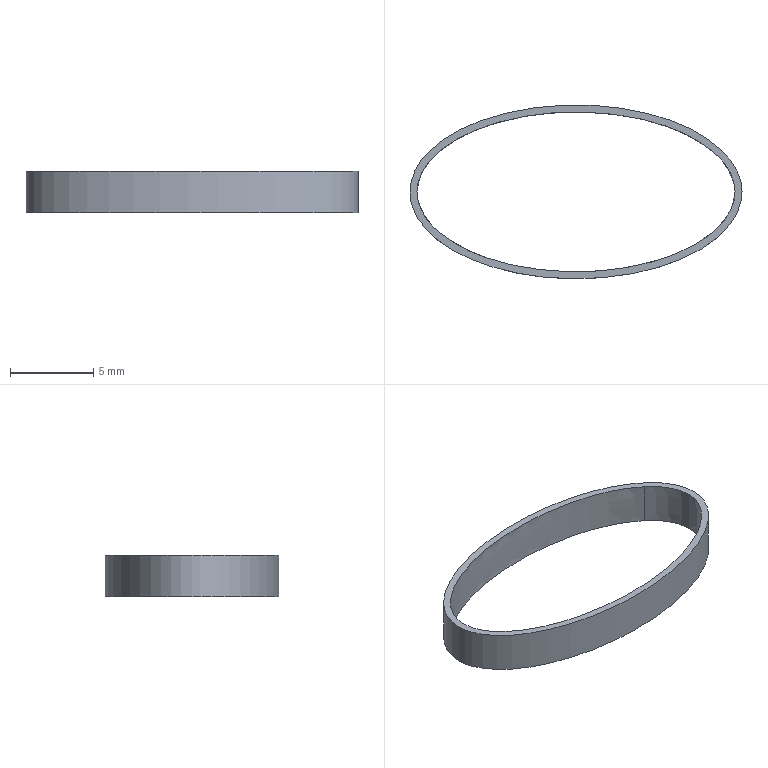Part | STEP file | lll_id1110_x_t | 1 solid | 9 faces | box 20 x 10.473 x 2.5 mm | volume 50.145 mm3 | other 7 | plane 2
STEP:
#1=CARTESIAN_POINT('',(381.689,-127.436,2.35));
#2=VERTEX_POINT('',#1);
#3=CARTESIAN_POINT('',(398.151,-127.436,2.35));
#4=VERTEX_POINT('',#3);
#5=CARTESIAN_POINT('',(381.689,-127.436,2.35));
#6=CARTESIAN_POINT('',(381.828,-127.553,2.35));
#7=CARTESIAN_POINT('',(381.971,-127.666,2.35));
#8=CARTESIAN_POINT('',(382.568,-128.082,2.35));
#9=CARTESIAN_POINT('',(383.043,-128.351,2.35));
#10=CARTESIAN_POINT('',(384.289,-128.906,2.35));
#11=CARTESIAN_POINT('',(385.064,-129.17,2.35));
#12=CARTESIAN_POINT('',(387.911,-129.83,2.35));
#13=CARTESIAN_POINT('',(390.012,-129.929,2.35));
#14=CARTESIAN_POINT('',(393.1,-129.572,2.35));
#15=CARTESIAN_POINT('',(394.082,-129.361,2.35));
#16=CARTESIAN_POINT('',(395.732,-128.839,2.35));
#17=CARTESIAN_POINT('',(396.4,-128.553,2.35));
#18=CARTESIAN_POINT('',(397.431,-127.982,2.35));
#19=CARTESIAN_POINT('',(397.804,-127.726,2.35));
#20=CARTESIAN_POINT('',(398.151,-127.436,2.35));
#21=(BOUNDED_CURVE()B_SPLINE_CURVE(3,(#5,#6,#7,#8,#9,#10,#11,#12,#13,#14,#15,#16,#17,#18,#19,#20),.UNSPECIFIED.,.F.,.F.)B_SPLINE_CURVE_WITH_KNOTS((4,2,2,2,2,2,2,4),(0.,0.03088,0.1235,0.2629,0.6224,0.7957,0.9214,1.),.UNSPECIFIED.)CURVE()GEOMETRIC_REPRESENTATION_ITEM()RATIONAL_B_SPLINE_CURVE((0.5011,0.5008,0.5008,0.4996,0.4996,0.4997,0.4997,0.4961,0.4961,0.4996,0.4996,0.4995,0.4995,0.4996,0.4996,0.5011))REPRESENTATION_ITEM(''));
#22=EDGE_CURVE('',#2,#4,#21,.T.);
#23=ORIENTED_EDGE('',*,*,#22,.T.);
#24=CARTESIAN_POINT('',(398.151,-127.436,-0.15));
#25=VERTEX_POINT('',#24);
#26=CARTESIAN_POINT('',(398.151,-127.436,-0.15));
#27=DIRECTION('',(0.,0.,1.));
#28=VECTOR('',#27,1.);
#29=LINE('',#26,#28);
#30=EDGE_CURVE('',#25,#4,#29,.T.);
#31=ORIENTED_EDGE('',*,*,#30,.F.);
#32=CARTESIAN_POINT('',(381.689,-127.436,-0.15));
#33=VERTEX_POINT('',#32);
#34=CARTESIAN_POINT('',(381.689,-127.436,-0.15));
#35=CARTESIAN_POINT('',(381.828,-127.553,-0.15));
#36=CARTESIAN_POINT('',(381.971,-127.666,-0.15));
#37=CARTESIAN_POINT('',(382.568,-128.082,-0.15));
#38=CARTESIAN_POINT('',(383.043,-128.351,-0.15));
#39=CARTESIAN_POINT('',(384.289,-128.906,-0.15));
#40=CARTESIAN_POINT('',(385.064,-129.17,-0.15));
#41=CARTESIAN_POINT('',(387.911,-129.83,-0.15));
#42=CARTESIAN_POINT('',(390.012,-129.929,-0.15));
#43=CARTESIAN_POINT('',(393.1,-129.572,-0.15));
#44=CARTESIAN_POINT('',(394.082,-129.361,-0.15));
#45=CARTESIAN_POINT('',(395.732,-128.839,-0.15));
#46=CARTESIAN_POINT('',(396.4,-128.553,-0.15));
#47=CARTESIAN_POINT('',(397.431,-127.982,-0.15));
#48=CARTESIAN_POINT('',(397.804,-127.726,-0.15));
#49=CARTESIAN_POINT('',(398.151,-127.436,-0.15));
#50=(BOUNDED_CURVE()B_SPLINE_CURVE(3,(#34,#35,#36,#37,#38,#39,#40,#41,#42,#43,#44,#45,#46,#47,#48,#49),.UNSPECIFIED.,.F.,.F.)B_SPLINE_CURVE_WITH_KNOTS((4,2,2,2,2,2,2,4),(0.,0.03088,0.1235,0.2629,0.6224,0.7957,0.9214,1.),.UNSPECIFIED.)CURVE()GEOMETRIC_REPRESENTATION_ITEM()RATIONAL_B_SPLINE_CURVE((0.5011,0.5008,0.5008,0.4996,0.4996,0.4997,0.4997,0.4961,0.4961,0.4996,0.4996,0.4995,0.4995,0.4996,0.4996,0.5011))REPRESENTATION_ITEM(''));
#51=EDGE_CURVE('',#33,#25,#50,.T.);
#52=ORIENTED_EDGE('',*,*,#51,.F.);
#53=CARTESIAN_POINT('',(381.689,-127.436,-0.15));
#54=DIRECTION('',(0.,0.,1.));
#55=VECTOR('',#54,1.);
#56=LINE('',#53,#55);
#57=EDGE_CURVE('',#33,#2,#56,.T.);
#58=ORIENTED_EDGE('',*,*,#57,.T.);
#59=EDGE_LOOP('',(#23,#31,#52,#58));
#60=FACE_OUTER_BOUND('',#59,.T.);
#61=CARTESIAN_POINT('',(381.689,-127.436,-0.15));
#62=CARTESIAN_POINT('',(381.828,-127.553,-0.15));
#63=CARTESIAN_POINT('',(381.971,-127.666,-0.15));
#64=CARTESIAN_POINT('',(382.568,-128.082,-0.15));
#65=CARTESIAN_POINT('',(383.043,-128.351,-0.15));
#66=CARTESIAN_POINT('',(384.289,-128.906,-0.15));
#67=CARTESIAN_POINT('',(385.064,-129.17,-0.15));
#68=CARTESIAN_POINT('',(387.911,-129.83,-0.15));
#69=CARTESIAN_POINT('',(390.012,-129.929,-0.15));
#70=CARTESIAN_POINT('',(393.1,-129.572,-0.15));
#71=CARTESIAN_POINT('',(394.082,-129.361,-0.15));
#72=CARTESIAN_POINT('',(395.732,-128.839,-0.15));
#73=CARTESIAN_POINT('',(396.4,-128.553,-0.15));
#74=CARTESIAN_POINT('',(397.431,-127.982,-0.15));
#75=CARTESIAN_POINT('',(397.804,-127.726,-0.15));
#76=CARTESIAN_POINT('',(398.151,-127.436,-0.15));
#77=(BOUNDED_CURVE()B_SPLINE_CURVE(3,(#61,#62,#63,#64,#65,#66,#67,#68,#69,#70,#71,#72,#73,#74,#75,#76),.UNSPECIFIED.,.F.,.F.)B_SPLINE_CURVE_WITH_KNOTS((4,2,2,2,2,2,2,4),(0.,0.03088,0.1235,0.2629,0.6224,0.7957,0.9214,1.),.UNSPECIFIED.)CURVE()GEOMETRIC_REPRESENTATION_ITEM()RATIONAL_B_SPLINE_CURVE((0.5011,0.5008,0.5008,0.4996,0.4996,0.4997,0.4997,0.4961,0.4961,0.4996,0.4996,0.4995,0.4995,0.4996,0.4996,0.5011))REPRESENTATION_ITEM(''));
#78=DIRECTION('',(0.,0.,1.));
#79=VECTOR('',#78,1.);
#80=SURFACE_OF_LINEAR_EXTRUSION('',#77,#79);
#81=ADVANCED_FACE('',(#60),#80,.F.);
#82=CARTESIAN_POINT('',(399.5,-125.,2.35));
#83=VERTEX_POINT('',#82);
#84=CARTESIAN_POINT('',(398.151,-127.436,2.35));
#85=CARTESIAN_POINT('',(398.314,-127.299,2.35));
#86=CARTESIAN_POINT('',(398.468,-127.152,2.35));
#87=CARTESIAN_POINT('',(398.795,-126.801,2.35));
#88=CARTESIAN_POINT('',(398.957,-126.589,2.35));
#89=CARTESIAN_POINT('',(399.188,-126.208,2.35));
#90=CARTESIAN_POINT('',(399.266,-126.048,2.35));
#91=CARTESIAN_POINT('',(399.443,-125.601,2.35));
#92=CARTESIAN_POINT('',(399.499,-125.303,2.35));
#93=CARTESIAN_POINT('',(399.5,-125.,2.35));
#94=(BOUNDED_CURVE()B_SPLINE_CURVE(3,(#84,#85,#86,#87,#88,#89,#90,#91,#92,#93),.UNSPECIFIED.,.F.,.F.)B_SPLINE_CURVE_WITH_KNOTS((4,2,2,2,4),(0.,0.2207,0.498,0.6834,1.),.UNSPECIFIED.)CURVE()GEOMETRIC_REPRESENTATION_ITEM()RATIONAL_B_SPLINE_CURVE((0.5044,0.5037,0.5037,0.5027,0.5027,0.5031,0.5031,0.4985,0.4985,0.5044))REPRESENTATION_ITEM(''));
#95=EDGE_CURVE('',#4,#83,#94,.T.);
#96=ORIENTED_EDGE('',*,*,#95,.T.);
#97=CARTESIAN_POINT('',(399.5,-125.,-0.15));
#98=VERTEX_POINT('',#97);
#99=CARTESIAN_POINT('',(399.5,-125.,-0.15));
#100=DIRECTION('',(0.,0.,1.));
#101=VECTOR('',#100,1.);
#102=LINE('',#99,#101);
#103=EDGE_CURVE('',#98,#83,#102,.T.);
#104=ORIENTED_EDGE('',*,*,#103,.F.);
#105=CARTESIAN_POINT('',(398.151,-127.436,-0.15));
#106=CARTESIAN_POINT('',(398.314,-127.299,-0.15));
#107=CARTESIAN_POINT('',(398.468,-127.152,-0.15));
#108=CARTESIAN_POINT('',(398.795,-126.801,-0.15));
#109=CARTESIAN_POINT('',(398.957,-126.589,-0.15));
#110=CARTESIAN_POINT('',(399.188,-126.208,-0.15));
#111=CARTESIAN_POINT('',(399.266,-126.048,-0.15));
#112=CARTESIAN_POINT('',(399.443,-125.601,-0.15));
#113=CARTESIAN_POINT('',(399.499,-125.303,-0.15));
#114=CARTESIAN_POINT('',(399.5,-125.,-0.15));
#115=(BOUNDED_CURVE()B_SPLINE_CURVE(3,(#105,#106,#107,#108,#109,#110,#111,#112,#113,#114),.UNSPECIFIED.,.F.,.F.)B_SPLINE_CURVE_WITH_KNOTS((4,2,2,2,4),(0.,0.2207,0.498,0.6834,1.),.UNSPECIFIED.)CURVE()GEOMETRIC_REPRESENTATION_ITEM()RATIONAL_B_SPLINE_CURVE((0.5044,0.5037,0.5037,0.5027,0.5027,0.5031,0.5031,0.4985,0.4985,0.5044))REPRESENTATION_ITEM(''));
#116=EDGE_CURVE('',#25,#98,#115,.T.);
#117=ORIENTED_EDGE('',*,*,#116,.F.);
#118=ORIENTED_EDGE('',*,*,#30,.T.);
#119=EDGE_LOOP('',(#96,#104,#117,#118));
#120=FACE_OUTER_BOUND('',#119,.T.);
#121=CARTESIAN_POINT('',(398.151,-127.436,-0.15));
#122=CARTESIAN_POINT('',(398.314,-127.299,-0.15));
#123=CARTESIAN_POINT('',(398.468,-127.152,-0.15));
#124=CARTESIAN_POINT('',(398.795,-126.801,-0.15));
#125=CARTESIAN_POINT('',(398.957,-126.589,-0.15));
#126=CARTESIAN_POINT('',(399.188,-126.208,-0.15));
#127=CARTESIAN_POINT('',(399.266,-126.048,-0.15));
#128=CARTESIAN_POINT('',(399.443,-125.601,-0.15));
#129=CARTESIAN_POINT('',(399.499,-125.303,-0.15));
#130=CARTESIAN_POINT('',(399.5,-125.,-0.15));
#131=(BOUNDED_CURVE()B_SPLINE_CURVE(3,(#121,#122,#123,#124,#125,#126,#127,#128,#129,#130),.UNSPECIFIED.,.F.,.F.)B_SPLINE_CURVE_WITH_KNOTS((4,2,2,2,4),(0.,0.2207,0.498,0.6834,1.),.UNSPECIFIED.)CURVE()GEOMETRIC_REPRESENTATION_ITEM()RATIONAL_B_SPLINE_CURVE((0.5044,0.5037,0.5037,0.5027,0.5027,0.5031,0.5031,0.4985,0.4985,0.5044))REPRESENTATION_ITEM(''));
#132=DIRECTION('',(0.,0.,1.));
#133=VECTOR('',#132,1.);
#134=SURFACE_OF_LINEAR_EXTRUSION('',#131,#133);
#135=ADVANCED_FACE('',(#120),#134,.F.);
#136=CARTESIAN_POINT('',(398.151,-122.564,2.35));
#137=VERTEX_POINT('',#136);
#138=CARTESIAN_POINT('',(399.5,-125.,2.35));
#139=CARTESIAN_POINT('',(399.499,-124.667,2.35));
#140=CARTESIAN_POINT('',(399.429,-124.341,2.35));
#141=CARTESIAN_POINT('',(399.24,-123.898,2.35));
#142=CARTESIAN_POINT('',(399.172,-123.766,2.35));
#143=CARTESIAN_POINT('',(398.972,-123.437,2.35));
#144=CARTESIAN_POINT('',(398.831,-123.247,2.35));
#145=CARTESIAN_POINT('',(398.512,-122.889,2.35));
#146=CARTESIAN_POINT('',(398.337,-122.72,2.35));
#147=CARTESIAN_POINT('',(398.151,-122.564,2.35));
#148=(BOUNDED_CURVE()B_SPLINE_CURVE(3,(#138,#139,#140,#141,#142,#143,#144,#145,#146,#147),.UNSPECIFIED.,.F.,.F.)B_SPLINE_CURVE_WITH_KNOTS((4,2,2,2,4),(0.,0.3431,0.4977,0.7454,1.),.UNSPECIFIED.)CURVE()GEOMETRIC_REPRESENTATION_ITEM()RATIONAL_B_SPLINE_CURVE((0.5007,0.4938,0.4938,0.4998,0.4998,0.4993,0.4993,0.4998,0.4998,0.5007))REPRESENTATION_ITEM(''));
#149=EDGE_CURVE('',#83,#137,#148,.T.);
#150=ORIENTED_EDGE('',*,*,#149,.T.);
#151=CARTESIAN_POINT('',(398.151,-122.564,-0.15));
#152=VERTEX_POINT('',#151);
#153=CARTESIAN_POINT('',(398.151,-122.564,-0.15));
#154=DIRECTION('',(0.,0.,1.));
#155=VECTOR('',#154,1.);
#156=LINE('',#153,#155);
#157=EDGE_CURVE('',#152,#137,#156,.T.);
#158=ORIENTED_EDGE('',*,*,#157,.F.);
#159=CARTESIAN_POINT('',(399.5,-125.,-0.15));
#160=CARTESIAN_POINT('',(399.499,-124.667,-0.15));
#161=CARTESIAN_POINT('',(399.429,-124.341,-0.15));
#162=CARTESIAN_POINT('',(399.24,-123.898,-0.15));
#163=CARTESIAN_POINT('',(399.172,-123.766,-0.15));
#164=CARTESIAN_POINT('',(398.972,-123.437,-0.15));
#165=CARTESIAN_POINT('',(398.831,-123.247,-0.15));
#166=CARTESIAN_POINT('',(398.512,-122.889,-0.15));
#167=CARTESIAN_POINT('',(398.337,-122.72,-0.15));
#168=CARTESIAN_POINT('',(398.151,-122.564,-0.15));
#169=(BOUNDED_CURVE()B_SPLINE_CURVE(3,(#159,#160,#161,#162,#163,#164,#165,#166,#167,#168),.UNSPECIFIED.,.F.,.F.)B_SPLINE_CURVE_WITH_KNOTS((4,2,2,2,4),(0.,0.3431,0.4977,0.7454,1.),.UNSPECIFIED.)CURVE()GEOMETRIC_REPRESENTATION_ITEM()RATIONAL_B_SPLINE_CURVE((0.5007,0.4938,0.4938,0.4998,0.4998,0.4993,0.4993,0.4998,0.4998,0.5007))REPRESENTATION_ITEM(''));
#170=EDGE_CURVE('',#98,#152,#169,.T.);
#171=ORIENTED_EDGE('',*,*,#170,.F.);
#172=ORIENTED_EDGE('',*,*,#103,.T.);
#173=EDGE_LOOP('',(#150,#158,#171,#172));
#174=FACE_OUTER_BOUND('',#173,.T.);
#175=CARTESIAN_POINT('',(399.5,-125.,-0.15));
#176=CARTESIAN_POINT('',(399.499,-124.667,-0.15));
#177=CARTESIAN_POINT('',(399.429,-124.341,-0.15));
#178=CARTESIAN_POINT('',(399.24,-123.898,-0.15));
#179=CARTESIAN_POINT('',(399.172,-123.766,-0.15));
#180=CARTESIAN_POINT('',(398.972,-123.437,-0.15));
#181=CARTESIAN_POINT('',(398.831,-123.247,-0.15));
#182=CARTESIAN_POINT('',(398.512,-122.889,-0.15));
#183=CARTESIAN_POINT('',(398.337,-122.72,-0.15));
#184=CARTESIAN_POINT('',(398.151,-122.564,-0.15));
#185=(BOUNDED_CURVE()B_SPLINE_CURVE(3,(#175,#176,#177,#178,#179,#180,#181,#182,#183,#184),.UNSPECIFIED.,.F.,.F.)B_SPLINE_CURVE_WITH_KNOTS((4,2,2,2,4),(0.,0.3431,0.4977,0.7454,1.),.UNSPECIFIED.)CURVE()GEOMETRIC_REPRESENTATION_ITEM()RATIONAL_B_SPLINE_CURVE((0.5007,0.4938,0.4938,0.4998,0.4998,0.4993,0.4993,0.4998,0.4998,0.5007))REPRESENTATION_ITEM(''));
#186=DIRECTION('',(0.,0.,1.));
#187=VECTOR('',#186,1.);
#188=SURFACE_OF_LINEAR_EXTRUSION('',#185,#187);
#189=ADVANCED_FACE('',(#174),#188,.F.);
#190=CARTESIAN_POINT('',(381.689,-122.564,2.35));
#191=VERTEX_POINT('',#190);
#192=CARTESIAN_POINT('',(398.151,-122.564,2.35));
#193=CARTESIAN_POINT('',(398.012,-122.447,2.35));
#194=CARTESIAN_POINT('',(397.869,-122.335,2.35));
#195=CARTESIAN_POINT('',(397.272,-121.918,2.35));
#196=CARTESIAN_POINT('',(396.797,-121.649,2.35));
#197=CARTESIAN_POINT('',(395.551,-121.094,2.35));
#198=CARTESIAN_POINT('',(394.776,-120.831,2.35));
#199=CARTESIAN_POINT('',(391.929,-120.17,2.35));
#200=CARTESIAN_POINT('',(389.828,-120.071,2.35));
#201=CARTESIAN_POINT('',(386.74,-120.428,2.35));
#202=CARTESIAN_POINT('',(385.758,-120.639,2.35));
#203=CARTESIAN_POINT('',(384.108,-121.162,2.35));
#204=CARTESIAN_POINT('',(383.44,-121.447,2.35));
#205=CARTESIAN_POINT('',(382.409,-122.018,2.35));
#206=CARTESIAN_POINT('',(382.036,-122.274,2.35));
#207=CARTESIAN_POINT('',(381.689,-122.564,2.35));
#208=(BOUNDED_CURVE()B_SPLINE_CURVE(3,(#192,#193,#194,#195,#196,#197,#198,#199,#200,#201,#202,#203,#204,#205,#206,#207),.UNSPECIFIED.,.F.,.F.)B_SPLINE_CURVE_WITH_KNOTS((4,2,2,2,2,2,2,4),(0.,0.03088,0.1235,0.2629,0.6224,0.7957,0.9214,1.),.UNSPECIFIED.)CURVE()GEOMETRIC_REPRESENTATION_ITEM()RATIONAL_B_SPLINE_CURVE((0.5011,0.5008,0.5008,0.4996,0.4996,0.4997,0.4997,0.4961,0.4961,0.4996,0.4996,0.4995,0.4995,0.4996,0.4996,0.5011))REPRESENTATION_ITEM(''));
#209=EDGE_CURVE('',#137,#191,#208,.T.);
#210=ORIENTED_EDGE('',*,*,#209,.T.);
#211=CARTESIAN_POINT('',(381.689,-122.564,-0.15));
#212=VERTEX_POINT('',#211);
#213=CARTESIAN_POINT('',(381.689,-122.564,-0.15));
#214=DIRECTION('',(0.,0.,1.));
#215=VECTOR('',#214,1.);
#216=LINE('',#213,#215);
#217=EDGE_CURVE('',#212,#191,#216,.T.);
#218=ORIENTED_EDGE('',*,*,#217,.F.);
#219=CARTESIAN_POINT('',(398.151,-122.564,-0.15));
#220=CARTESIAN_POINT('',(398.012,-122.447,-0.15));
#221=CARTESIAN_POINT('',(397.869,-122.335,-0.15));
#222=CARTESIAN_POINT('',(397.272,-121.918,-0.15));
#223=CARTESIAN_POINT('',(396.797,-121.649,-0.15));
#224=CARTESIAN_POINT('',(395.551,-121.094,-0.15));
#225=CARTESIAN_POINT('',(394.776,-120.831,-0.15));
#226=CARTESIAN_POINT('',(391.929,-120.17,-0.15));
#227=CARTESIAN_POINT('',(389.828,-120.071,-0.15));
#228=CARTESIAN_POINT('',(386.74,-120.428,-0.15));
#229=CARTESIAN_POINT('',(385.758,-120.639,-0.15));
#230=CARTESIAN_POINT('',(384.108,-121.162,-0.15));
#231=CARTESIAN_POINT('',(383.44,-121.447,-0.15));
#232=CARTESIAN_POINT('',(382.409,-122.018,-0.15));
#233=CARTESIAN_POINT('',(382.036,-122.274,-0.15));
#234=CARTESIAN_POINT('',(381.689,-122.564,-0.15));
#235=(BOUNDED_CURVE()B_SPLINE_CURVE(3,(#219,#220,#221,#222,#223,#224,#225,#226,#227,#228,#229,#230,#231,#232,#233,#234),.UNSPECIFIED.,.F.,.F.)B_SPLINE_CURVE_WITH_KNOTS((4,2,2,2,2,2,2,4),(0.,0.03088,0.1235,0.2629,0.6224,0.7957,0.9214,1.),.UNSPECIFIED.)CURVE()GEOMETRIC_REPRESENTATION_ITEM()RATIONAL_B_SPLINE_CURVE((0.5011,0.5008,0.5008,0.4996,0.4996,0.4997,0.4997,0.4961,0.4961,0.4996,0.4996,0.4995,0.4995,0.4996,0.4996,0.5011))REPRESENTATION_ITEM(''));
#236=EDGE_CURVE('',#152,#212,#235,.T.);
#237=ORIENTED_EDGE('',*,*,#236,.F.);
#238=ORIENTED_EDGE('',*,*,#157,.T.);
#239=EDGE_LOOP('',(#210,#218,#237,#238));
#240=FACE_OUTER_BOUND('',#239,.T.);
#241=CARTESIAN_POINT('',(398.151,-122.564,-0.15));
#242=CARTESIAN_POINT('',(398.012,-122.447,-0.15));
#243=CARTESIAN_POINT('',(397.869,-122.335,-0.15));
#244=CARTESIAN_POINT('',(397.272,-121.918,-0.15));
#245=CARTESIAN_POINT('',(396.797,-121.649,-0.15));
#246=CARTESIAN_POINT('',(395.551,-121.094,-0.15));
#247=CARTESIAN_POINT('',(394.776,-120.831,-0.15));
#248=CARTESIAN_POINT('',(391.929,-120.17,-0.15));
#249=CARTESIAN_POINT('',(389.828,-120.071,-0.15));
#250=CARTESIAN_POINT('',(386.74,-120.428,-0.15));
#251=CARTESIAN_POINT('',(385.758,-120.639,-0.15));
#252=CARTESIAN_POINT('',(384.108,-121.162,-0.15));
#253=CARTESIAN_POINT('',(383.44,-121.447,-0.15));
#254=CARTESIAN_POINT('',(382.409,-122.018,-0.15));
#255=CARTESIAN_POINT('',(382.036,-122.274,-0.15));
#256=CARTESIAN_POINT('',(381.689,-122.564,-0.15));
#257=(BOUNDED_CURVE()B_SPLINE_CURVE(3,(#241,#242,#243,#244,#245,#246,#247,#248,#249,#250,#251,#252,#253,#254,#255,#256),.UNSPECIFIED.,.F.,.F.)B_SPLINE_CURVE_WITH_KNOTS((4,2,2,2,2,2,2,4),(0.,0.03088,0.1235,0.2629,0.6224,0.7957,0.9214,1.),.UNSPECIFIED.)CURVE()GEOMETRIC_REPRESENTATION_ITEM()RATIONAL_B_SPLINE_CURVE((0.5011,0.5008,0.5008,0.4996,0.4996,0.4997,0.4997,0.4961,0.4961,0.4996,0.4996,0.4995,0.4995,0.4996,0.4996,0.5011))REPRESENTATION_ITEM(''));
#258=DIRECTION('',(0.,0.,1.));
#259=VECTOR('',#258,1.);
#260=SURFACE_OF_LINEAR_EXTRUSION('',#257,#259);
#261=ADVANCED_FACE('',(#240),#260,.F.);
#262=CARTESIAN_POINT('',(380.34,-125.,2.35));
#263=VERTEX_POINT('',#262);
#264=CARTESIAN_POINT('',(381.689,-122.564,2.35));
#265=CARTESIAN_POINT('',(381.526,-122.701,2.35));
#266=CARTESIAN_POINT('',(381.372,-122.848,2.35));
#267=CARTESIAN_POINT('',(381.045,-123.199,2.35));
#268=CARTESIAN_POINT('',(380.883,-123.412,2.35));
#269=CARTESIAN_POINT('',(380.652,-123.792,2.35));
#270=CARTESIAN_POINT('',(380.574,-123.952,2.35));
#271=CARTESIAN_POINT('',(380.397,-124.399,2.35));
#272=CARTESIAN_POINT('',(380.341,-124.697,2.35));
#273=CARTESIAN_POINT('',(380.34,-125.,2.35));
#274=(BOUNDED_CURVE()B_SPLINE_CURVE(3,(#264,#265,#266,#267,#268,#269,#270,#271,#272,#273),.UNSPECIFIED.,.F.,.F.)B_SPLINE_CURVE_WITH_KNOTS((4,2,2,2,4),(0.,0.2207,0.498,0.6834,1.),.UNSPECIFIED.)CURVE()GEOMETRIC_REPRESENTATION_ITEM()RATIONAL_B_SPLINE_CURVE((0.5044,0.5037,0.5037,0.5027,0.5027,0.5031,0.5031,0.4985,0.4985,0.5044))REPRESENTATION_ITEM(''));
#275=EDGE_CURVE('',#191,#263,#274,.T.);
#276=ORIENTED_EDGE('',*,*,#275,.T.);
#277=CARTESIAN_POINT('',(380.34,-125.,-0.15));
#278=VERTEX_POINT('',#277);
#279=CARTESIAN_POINT('',(380.34,-125.,-0.15));
#280=DIRECTION('',(0.,0.,1.));
#281=VECTOR('',#280,1.);
#282=LINE('',#279,#281);
#283=EDGE_CURVE('',#278,#263,#282,.T.);
#284=ORIENTED_EDGE('',*,*,#283,.F.);
#285=CARTESIAN_POINT('',(381.689,-122.564,-0.15));
#286=CARTESIAN_POINT('',(381.526,-122.701,-0.15));
#287=CARTESIAN_POINT('',(381.372,-122.848,-0.15));
#288=CARTESIAN_POINT('',(381.045,-123.199,-0.15));
#289=CARTESIAN_POINT('',(380.883,-123.412,-0.15));
#290=CARTESIAN_POINT('',(380.652,-123.792,-0.15));
#291=CARTESIAN_POINT('',(380.574,-123.952,-0.15));
#292=CARTESIAN_POINT('',(380.397,-124.399,-0.15));
#293=CARTESIAN_POINT('',(380.341,-124.697,-0.15));
#294=CARTESIAN_POINT('',(380.34,-125.,-0.15));
#295=(BOUNDED_CURVE()B_SPLINE_CURVE(3,(#285,#286,#287,#288,#289,#290,#291,#292,#293,#294),.UNSPECIFIED.,.F.,.F.)B_SPLINE_CURVE_WITH_KNOTS((4,2,2,2,4),(0.,0.2207,0.498,0.6834,1.),.UNSPECIFIED.)CURVE()GEOMETRIC_REPRESENTATION_ITEM()RATIONAL_B_SPLINE_CURVE((0.5044,0.5037,0.5037,0.5027,0.5027,0.5031,0.5031,0.4985,0.4985,0.5044))REPRESENTATION_ITEM(''));
#296=EDGE_CURVE('',#212,#278,#295,.T.);
#297=ORIENTED_EDGE('',*,*,#296,.F.);
#298=ORIENTED_EDGE('',*,*,#217,.T.);
#299=EDGE_LOOP('',(#276,#284,#297,#298));
#300=FACE_OUTER_BOUND('',#299,.T.);
#301=CARTESIAN_POINT('',(381.689,-122.564,-0.15));
#302=CARTESIAN_POINT('',(381.526,-122.701,-0.15));
#303=CARTESIAN_POINT('',(381.372,-122.848,-0.15));
#304=CARTESIAN_POINT('',(381.045,-123.199,-0.15));
#305=CARTESIAN_POINT('',(380.883,-123.412,-0.15));
#306=CARTESIAN_POINT('',(380.652,-123.792,-0.15));
#307=CARTESIAN_POINT('',(380.574,-123.952,-0.15));
#308=CARTESIAN_POINT('',(380.397,-124.399,-0.15));
#309=CARTESIAN_POINT('',(380.341,-124.697,-0.15));
#310=CARTESIAN_POINT('',(380.34,-125.,-0.15));
#311=(BOUNDED_CURVE()B_SPLINE_CURVE(3,(#301,#302,#303,#304,#305,#306,#307,#308,#309,#310),.UNSPECIFIED.,.F.,.F.)B_SPLINE_CURVE_WITH_KNOTS((4,2,2,2,4),(0.,0.2207,0.498,0.6834,1.),.UNSPECIFIED.)CURVE()GEOMETRIC_REPRESENTATION_ITEM()RATIONAL_B_SPLINE_CURVE((0.5044,0.5037,0.5037,0.5027,0.5027,0.5031,0.5031,0.4985,0.4985,0.5044))REPRESENTATION_ITEM(''));
#312=DIRECTION('',(0.,0.,1.));
#313=VECTOR('',#312,1.);
#314=SURFACE_OF_LINEAR_EXTRUSION('',#311,#313);
#315=ADVANCED_FACE('',(#300),#314,.F.);
#316=CARTESIAN_POINT('',(379.92,-125.,2.35));
#317=VERTEX_POINT('',#316);
#318=CARTESIAN_POINT('',(389.92,-125.,2.35));
#319=DIRECTION('',(0.,0.,-1.));
#320=DIRECTION('',(-1.,0.,0.));
#321=AXIS2_PLACEMENT_3D('',#318,#319,#320);
#322=ELLIPSE('',#321,10.,5.236);
#323=EDGE_CURVE('',#317,#317,#322,.T.);
#324=ORIENTED_EDGE('',*,*,#323,.T.);
#325=EDGE_LOOP('',(#324));
#326=FACE_BOUND('',#325,.T.);
#327=CARTESIAN_POINT('',(379.92,-125.,-0.15));
#328=VERTEX_POINT('',#327);
#329=CARTESIAN_POINT('',(389.92,-125.,-0.15));
#330=DIRECTION('',(0.,0.,-1.));
#331=DIRECTION('',(-1.,0.,0.));
#332=AXIS2_PLACEMENT_3D('',#329,#330,#331);
#333=ELLIPSE('',#332,10.,5.236);
#334=EDGE_CURVE('',#328,#328,#333,.T.);
#335=ORIENTED_EDGE('',*,*,#334,.F.);
#336=EDGE_LOOP('',(#335));
#337=FACE_BOUND('',#336,.T.);
#338=CARTESIAN_POINT('',(389.92,-125.,-0.15));
#339=DIRECTION('',(0.,0.,-1.));
#340=DIRECTION('',(-1.,0.,0.));
#341=AXIS2_PLACEMENT_3D('',#338,#339,#340);
#342=ELLIPSE('',#341,10.,5.236);
#343=DIRECTION('',(0.,0.,1.));
#344=VECTOR('',#343,1.);
#345=SURFACE_OF_LINEAR_EXTRUSION('',#342,#344);
#346=ADVANCED_FACE('',(#326,#337),#345,.F.);
#347=CARTESIAN_POINT('',(380.34,-125.,2.35));
#348=CARTESIAN_POINT('',(380.341,-125.333,2.35));
#349=CARTESIAN_POINT('',(380.411,-125.659,2.35));
#350=CARTESIAN_POINT('',(380.6,-126.102,2.35));
#351=CARTESIAN_POINT('',(380.668,-126.234,2.35));
#352=CARTESIAN_POINT('',(380.868,-126.563,2.35));
#353=CARTESIAN_POINT('',(381.009,-126.753,2.35));
#354=CARTESIAN_POINT('',(381.328,-127.111,2.35));
#355=CARTESIAN_POINT('',(381.503,-127.28,2.35));
#356=CARTESIAN_POINT('',(381.689,-127.436,2.35));
#357=(BOUNDED_CURVE()B_SPLINE_CURVE(3,(#347,#348,#349,#350,#351,#352,#353,#354,#355,#356),.UNSPECIFIED.,.F.,.F.)B_SPLINE_CURVE_WITH_KNOTS((4,2,2,2,4),(0.,0.3431,0.4977,0.7454,1.),.UNSPECIFIED.)CURVE()GEOMETRIC_REPRESENTATION_ITEM()RATIONAL_B_SPLINE_CURVE((0.5007,0.4938,0.4938,0.4998,0.4998,0.4993,0.4993,0.4998,0.4998,0.5007))REPRESENTATION_ITEM(''));
#358=EDGE_CURVE('',#263,#2,#357,.T.);
#359=ORIENTED_EDGE('',*,*,#358,.T.);
#360=ORIENTED_EDGE('',*,*,#57,.F.);
#361=CARTESIAN_POINT('',(380.34,-125.,-0.15));
#362=CARTESIAN_POINT('',(380.341,-125.333,-0.15));
#363=CARTESIAN_POINT('',(380.411,-125.659,-0.15));
#364=CARTESIAN_POINT('',(380.6,-126.102,-0.15));
#365=CARTESIAN_POINT('',(380.668,-126.234,-0.15));
#366=CARTESIAN_POINT('',(380.868,-126.563,-0.15));
#367=CARTESIAN_POINT('',(381.009,-126.753,-0.15));
#368=CARTESIAN_POINT('',(381.328,-127.111,-0.15));
#369=CARTESIAN_POINT('',(381.503,-127.28,-0.15));
#370=CARTESIAN_POINT('',(381.689,-127.436,-0.15));
#371=(BOUNDED_CURVE()B_SPLINE_CURVE(3,(#361,#362,#363,#364,#365,#366,#367,#368,#369,#370),.UNSPECIFIED.,.F.,.F.)B_SPLINE_CURVE_WITH_KNOTS((4,2,2,2,4),(0.,0.3431,0.4977,0.7454,1.),.UNSPECIFIED.)CURVE()GEOMETRIC_REPRESENTATION_ITEM()RATIONAL_B_SPLINE_CURVE((0.5007,0.4938,0.4938,0.4998,0.4998,0.4993,0.4993,0.4998,0.4998,0.5007))REPRESENTATION_ITEM(''));
#372=EDGE_CURVE('',#278,#33,#371,.T.);
#373=ORIENTED_EDGE('',*,*,#372,.F.);
#374=ORIENTED_EDGE('',*,*,#283,.T.);
#375=EDGE_LOOP('',(#359,#360,#373,#374));
#376=FACE_OUTER_BOUND('',#375,.T.);
#377=CARTESIAN_POINT('',(380.34,-125.,-0.15));
#378=CARTESIAN_POINT('',(380.341,-125.333,-0.15));
#379=CARTESIAN_POINT('',(380.411,-125.659,-0.15));
#380=CARTESIAN_POINT('',(380.6,-126.102,-0.15));
#381=CARTESIAN_POINT('',(380.668,-126.234,-0.15));
#382=CARTESIAN_POINT('',(380.868,-126.563,-0.15));
#383=CARTESIAN_POINT('',(381.009,-126.753,-0.15));
#384=CARTESIAN_POINT('',(381.328,-127.111,-0.15));
#385=CARTESIAN_POINT('',(381.503,-127.28,-0.15));
#386=CARTESIAN_POINT('',(381.689,-127.436,-0.15));
#387=(BOUNDED_CURVE()B_SPLINE_CURVE(3,(#377,#378,#379,#380,#381,#382,#383,#384,#385,#386),.UNSPECIFIED.,.F.,.F.)B_SPLINE_CURVE_WITH_KNOTS((4,2,2,2,4),(0.,0.3431,0.4977,0.7454,1.),.UNSPECIFIED.)CURVE()GEOMETRIC_REPRESENTATION_ITEM()RATIONAL_B_SPLINE_CURVE((0.5007,0.4938,0.4938,0.4998,0.4998,0.4993,0.4993,0.4998,0.4998,0.5007))REPRESENTATION_ITEM(''));
#388=DIRECTION('',(0.,0.,1.));
#389=VECTOR('',#388,1.);
#390=SURFACE_OF_LINEAR_EXTRUSION('',#387,#389);
#391=ADVANCED_FACE('',(#376),#390,.F.);
#392=ORIENTED_EDGE('',*,*,#334,.T.);
#393=EDGE_LOOP('',(#392));
#394=FACE_BOUND('',#393,.T.);
#395=ORIENTED_EDGE('',*,*,#51,.T.);
#396=ORIENTED_EDGE('',*,*,#116,.T.);
#397=ORIENTED_EDGE('',*,*,#170,.T.);
#398=ORIENTED_EDGE('',*,*,#236,.T.);
#399=ORIENTED_EDGE('',*,*,#296,.T.);
#400=ORIENTED_EDGE('',*,*,#372,.T.);
#401=EDGE_LOOP('',(#395,#396,#397,#398,#399,#400));
#402=FACE_BOUND('',#401,.T.);
#403=CARTESIAN_POINT('',(389.92,-125.,-0.15));
#404=DIRECTION('',(0.,0.,-1.));
#405=DIRECTION('',(-1.,0.,0.));
#406=AXIS2_PLACEMENT_3D('',#403,#404,#405);
#407=PLANE('',#406);
#408=ADVANCED_FACE('',(#394,#402),#407,.T.);
#409=ORIENTED_EDGE('',*,*,#323,.F.);
#410=EDGE_LOOP('',(#409));
#411=FACE_BOUND('',#410,.T.);
#412=ORIENTED_EDGE('',*,*,#22,.F.);
#413=ORIENTED_EDGE('',*,*,#358,.F.);
#414=ORIENTED_EDGE('',*,*,#275,.F.);
#415=ORIENTED_EDGE('',*,*,#209,.F.);
#416=ORIENTED_EDGE('',*,*,#149,.F.);
#417=ORIENTED_EDGE('',*,*,#95,.F.);
#418=EDGE_LOOP('',(#412,#413,#414,#415,#416,#417));
#419=FACE_BOUND('',#418,.T.);
#420=CARTESIAN_POINT('',(389.92,-125.,2.35));
#421=DIRECTION('',(0.,0.,-1.));
#422=DIRECTION('',(-1.,0.,0.));
#423=AXIS2_PLACEMENT_3D('',#420,#421,#422);
#424=PLANE('',#423);
#425=ADVANCED_FACE('',(#411,#419),#424,.F.);
#426=CLOSED_SHELL('',(#81,#135,#189,#261,#315,#346,#391,#408,#425));
#427=MANIFOLD_SOLID_BREP('',#426);
#428=(LENGTH_UNIT()NAMED_UNIT(*)SI_UNIT(.MILLI.,.METRE.));
#429=UNCERTAINTY_MEASURE_WITH_UNIT(LENGTH_MEASURE(0.00002),#428,'','');
#430=(NAMED_UNIT(*)PLANE_ANGLE_UNIT()SI_UNIT($,.RADIAN.));
#431=PLANE_ANGLE_MEASURE_WITH_UNIT(PLANE_ANGLE_MEASURE(0.01745),#430);
#432=DIMENSIONAL_EXPONENTS(0.,0.,0.,0.,0.,0.,0.);
#433=(CONVERSION_BASED_UNIT('DEGREE',#431)NAMED_UNIT(#432)PLANE_ANGLE_UNIT());
#434=(NAMED_UNIT(*)SI_UNIT($,.STERADIAN.)SOLID_ANGLE_UNIT());
#435=(GEOMETRIC_REPRESENTATION_CONTEXT(3)GLOBAL_UNCERTAINTY_ASSIGNED_CONTEXT((#429))GLOBAL_UNIT_ASSIGNED_CONTEXT((#428,#433,#434))REPRESENTATION_CONTEXT('',''));
#436=ADVANCED_BREP_SHAPE_REPRESENTATION('',(#427),#435);